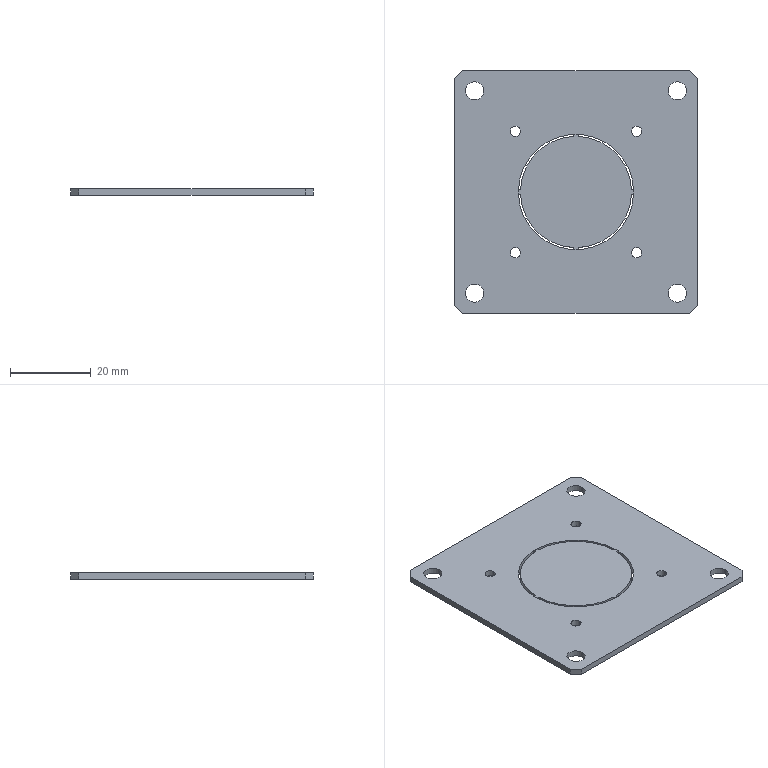Part | STEP file | JK-Aviation plug | 2 solids | 46 faces | box 60 x 60 x 1.5 mm | volume 5200 mm3 | plane 24 | cylinder 22 | commonest cylinder face diameters 2.5 x8 4.5 x8 27.5 x4 28.5 x2